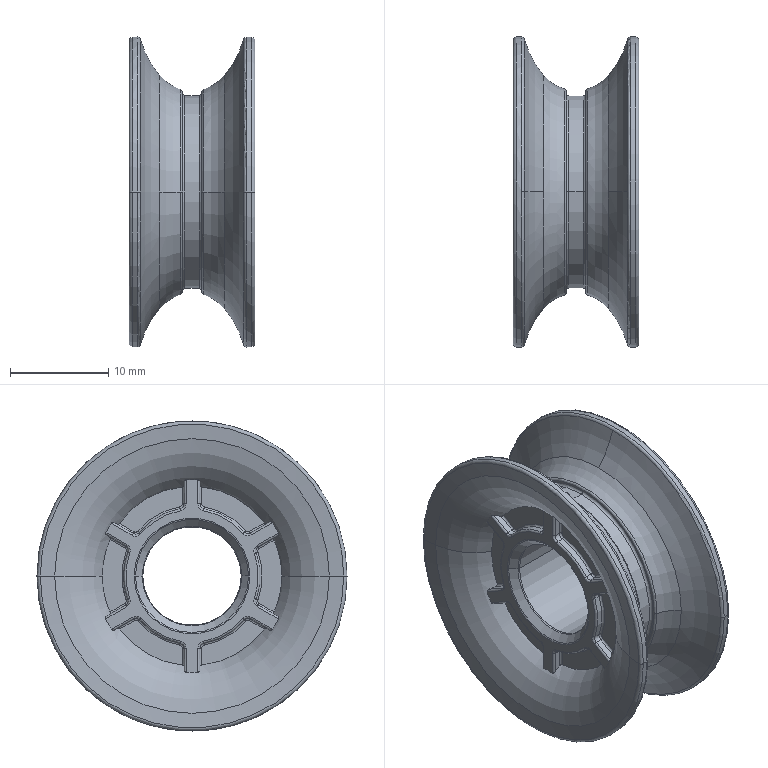Part | STEP file | MSBR-24 | 1 solid | 244 faces | box 12.744 x 31.5 x 31.5 mm | volume 3459 mm3 | torus 82 | cylinder 80 | plane 40 | spline 24 | cone 18 | commonest cylinder face diameters 0.4 x48 1 x24 31.5 x4 10 x2 19.6 x2